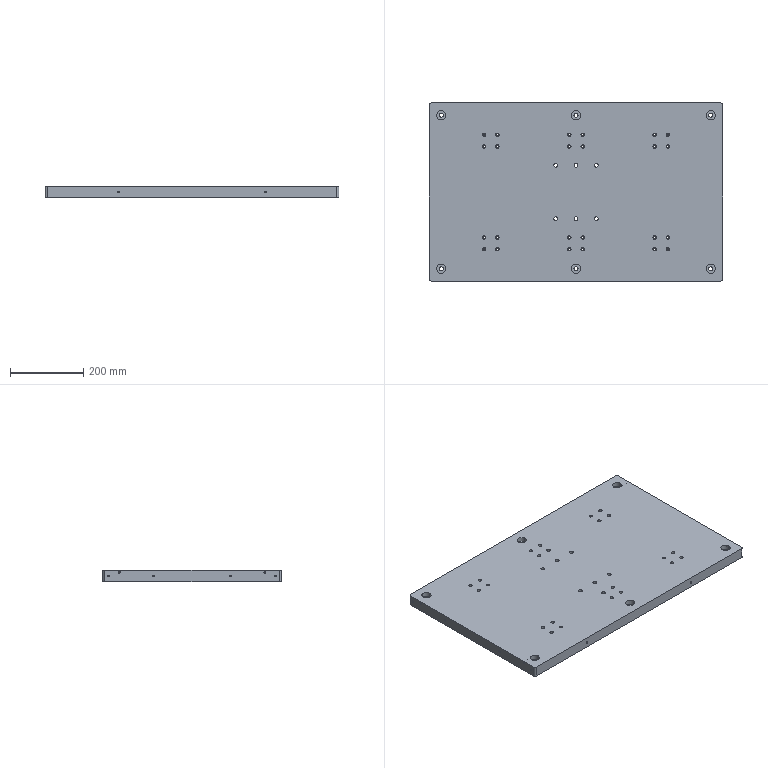CAM job | Mastercam | 3-axis milling, drilling | part box 800 x 485 x 30 mm
Tools:
tool_number,name,type,diameter_mm,corner_radius_mm,flutes,flute_length_mm,overall_length_mm,shoulder_length_mm,holder_diameter_mm,length_offset,diameter_offset,default_rpm,default_feed_mm_min,default_plunge_mm_min,coolant
1,11 Drill,drill,11,0,2,25,50,40,50,1,1,545,65.4,600,COOL_OFF
1,6.8 Drill,drill,6.8,0,2,25,50,40,50,1,1,1500,200,600,COOL_OFF
1,11 Drill,drill,11,0,2,25,50,40,50,1,1,545,65.4,600,COOL_OFF
1,11 Drill,drill,11,0,2,25,50,40,50,1,1,545,65.4,600,COOL_OFF
1,10 Drill,drill,10,0,2,25,50,40,50,1,1,600,72,600,COOL_OFF
5,5 Flat End Mill,end mill,5,0,4,25,75,25,50,5,5,2000,240,600,COOL_OFF
7,4 Chamfer Mill,chamfer mill,4,0,4,25,75,30,50,7,7,6250,750,600,COOL_OFF
7,6 Chamfer Mill,chamfer mill,6,0,4,25,75,30,50,7,7,7000,1000,600,COOL_OFF
7,4 Chamfer Mill,chamfer mill,4,0,4,25,75,30,50,7,7,6250,750,600,COOL_OFF
7,4 Chamfer Mill,chamfer mill,4,0,4,25,75,30,50,7,7,6250,750,600,COOL_OFF
9,10 Flat End Mill,end mill,10,0,4,25,75,25,50,9,9,1000,120,600,COOL_OFF
9,10 Flat End Mill,end mill,10,0,4,25,75,25,50,9,9,7000,3000,600,COOL_OFF
9,10 Flat End Mill,end mill,10,0,4,25,75,25,50,9,9,1000,120,600,COOL_OFF
9,10 Flat End Mill,end mill,10,0,4,25,75,25,50,9,9,1000,120,600,COOL_OFF
10,10 Flat End Mill,end mill,10,0,4,25,75,25,50,10,10,1000,120,600,COOL_OFF
10,10 Flat End Mill,end mill,10,0,4,25,75,25,50,10,10,1000,120,600,COOL_OFF
10,10 Flat End Mill,end mill,10,0,4,25,75,25,50,10,10,7000,1000,600,COOL_OFF
10,10 Flat End Mill,end mill,10,0,4,25,75,25,50,10,10,1000,120,600,COOL_OFF
14,10.5 Drill,drill,10.5,0,2,25,50,40,50,14,14,571,68.52,600,COOL_OFF
14,10.5 Drill,drill,10.5,0,2,25,50,40,50,14,14,571,68.52,600,COOL_OFF
14,10.5 Drill,drill,10.5,0,2,25,50,40,50,14,14,571,68.52,600,COOL_OFF
15,5.5 Drill,drill,5.5,0,2,25,50,40,50,15,15,1091,130.92,600,COOL_OFF
18,8 Drill,drill,8,0,2,25,50,40,50,18,18,1400,200,600,COOL_OFF
18,5.1 Drill,drill,5.1,0,2,25,50,40,50,18,18,1176,141.12,600,COOL_OFF
18,5.1 Drill,drill,5.1,0,2,25,50,40,50,18,18,1176,141.12,600,COOL_OFF
18,8.5 Drill,drill,8.5,0,2,25,50,40,50,18,18,706,84.72,600,COOL_OFF
19,9 Drill,drill,9,0,2,25,50,40,50,19,19,666,79.92,600,COOL_OFF
20,20 Flat End Mill,end mill,20,0,4,25,75,25,50,20,20,500,60,600,COOL_OFF
20,20 Flat End Mill,end mill,20,0,4,25,75,25,50,20,20,5000,4000,600,COOL_OFF
20,20 Flat End Mill,end mill,20,0,4,25,75,25,50,20,20,500,60,600,COOL_OFF
20,20 Flat End Mill,end mill,20,0,4,25,75,25,50,20,20,500,60,600,COOL_OFF
24,100 Flat End Mill,end mill,100,0,4,25,75,25,50,24,24,100,12,600,COOL_OFF
Operations:
seq,operation,operation_type,tool_number,tool_name,tool_diameter_mm,spindle_rpm,feed_mm_min,plunge_mm_min,retract_mm_min,cycle_time_s,wcs,posted,nc_file
1,Manual Entry (clamp x),ManualEntry,,,,0,0,0,0,0,Plane-1,yes,1.nc
2,Contour (Ramp) - [WCS: Plane-1] - [Tplane: Plane-1],Contour,20,20 Flat End Mill,20,5000,4000,600,1200,754.428,Plane-1,yes,1.nc
3,Contour (2D) - [WCS: Plane-1] - [Tplane: Plane-1],Contour,20,20 Flat End Mill,20,5000,1000,600,1200,221.553,Plane-1,yes,1.nc
4,Contour (2D chamfer) - [WCS: Plane-1] - [Tplane: Plane-1],Contour,7,4 Chamfer Mill,4,6500,1000,600,1200,98.508,Plane-1,yes,1.nc
5,Manual Entry (cCl，cy),ManualEntry,,,,0,0,0,0,0,Plane-1,yes,1.nc
6,Manual Entry (M00),ManualEntry,,,,0,0,0,0,0,Plane-1,yes,1.nc
7,Contour (Ramp) - [WCS: Plane-1] - [Tplane: Plane-1],Contour,20,20 Flat End Mill,20,5000,4000,600,1200,486.877,Plane-1,yes,1.nc
8,Contour (2D) - [WCS: Plane-1] - [Tplane: Plane-1],Contour,20,20 Flat End Mill,20,5000,1000,600,1200,147.1,Plane-1,yes,1.nc
9,Contour (2D chamfer) - [WCS: Plane-1] - [Tplane: Plane-1],Contour,7,4 Chamfer Mill,4,6500,1000,600,1200,60.684,Plane-1,yes,1.nc
10,Manual Entry (X+Cl),ManualEntry,,,,0,0,0,0,0,Plane-1,yes,1.nc
11,Manual Entry (M00),ManualEntry,,,,0,0,0,0,0,Plane-1,yes,1.nc
12,Drill/Counterbore - [WCS: Plane-1] - [Tplane: Plane-1],Drill,7,4 Chamfer Mill,4,6000,200,600,1200,35.588,Plane-1,yes,1.nc
13,Peck Drill - [WCS: Plane-1] - [Tplane: Plane-1],Drill,1,10 Drill,10,800,80,600,1200,156.133,Plane-1,yes,1.nc
14,Peck Drill - [WCS: Plane-1] - [Tplane: Plane-1],Drill,15,5.5 Drill,5.5,1200,120,600,1200,439.734,Plane-1,yes,1.nc
15,Peck Drill - [WCS: Plane-1] - [Tplane: Plane-1],Drill,14,10.5 Drill,10.5,800,100,600,1200,128.413,Plane-1,yes,1.nc
16,Helix Bore - [WCS: Plane-1] - [Tplane: Plane-1],HelixBore,5,5 Flat End Mill,5,6500,2000,600,1200,485.706,Plane-1,yes,1.nc
17,Contour (Ramp) - [WCS: Plane-1] - [Tplane: Plane-1],Contour,9,10 Flat End Mill,10,6500,3000,600,1200,113.28,Plane-1,yes,1.nc
18,Contour (2D) - [WCS: Plane-1] - [Tplane: Plane-1],Contour,10,10 Flat End Mill,10,6500,1000,600,1200,59.619,Plane-1,yes,1.nc
19,Contour (2D chamfer) - [WCS: Plane-1] - [Tplane: Plane-1],Contour,7,4 Chamfer Mill,4,6000,1000,600,1200,116.625,Plane-1,yes,1.nc
20,Contour (Ramp) - [WCS: Plane-2] - [Tplane: Plane-2],Contour,9,10 Flat End Mill,10,6500,2000,600,1200,80.577,Plane-2,yes,1.nc
21,Contour (2D) - [WCS: Plane-2] - [Tplane: Plane-2],Contour,10,10 Flat End Mill,10,6500,1000,600,1200,19.005,Plane-2,yes,1.nc
22,Contour (2D chamfer) - [WCS: Plane-2] - [Tplane: Plane-2],Contour,7,4 Chamfer Mill,4,6000,1000,600,1200,37.556,Plane-2,yes,1.nc
23,Drill/Counterbore - [WCS: Plane-3] - [Tplane: Plane-3],Drill,7,4 Chamfer Mill,4,6000,200,600,1200,1.977,Plane-3,yes,1.nc
24,Peck Drill - [WCS: Plane-3] - [Tplane: Plane-3],Drill,18,8.5 Drill,8.5,1200,100,600,1200,31.296,Plane-3,yes,1.nc
25,Contour (2D chamfer) - [WCS: Plane-3] - [Tplane: Plane-3],Contour,7,4 Chamfer Mill,4,6000,1000,600,1200,3.002,Plane-3,yes,1.nc
26,Drill/Counterbore - [WCS: Plane-4] - [Tplane: Plane-4],Drill,7,4 Chamfer Mill,4,6000,200,600,1200,5.931,Plane-4,yes,1.nc
27,Peck Drill - [WCS: Plane-4] - [Tplane: Plane-4],Drill,15,5.5 Drill,5.5,1200,100,600,1200,85.363,Plane-4,yes,1.nc
28,Contour (2D chamfer) - [WCS: Plane-4] - [Tplane: Plane-4],Contour,7,4 Chamfer Mill,4,6000,1000,600,1200,9.231,Plane-4,yes,1.nc
29,Contour (Ramp) - [WCS: Plane-2] - [Tplane: Plane-2],Contour,10,10 Flat End Mill,10,6500,1500,600,1200,29.736,Plane-2,yes,1.nc
30,Manual Entry (clamp x),ManualEntry,,,,0,0,0,0,0,Plane-5,yes,4.nc
31,Contour (Ramp) - [WCS: Plane-5] - [Tplane: Plane-5],Contour,20,20 Flat End Mill,20,5000,4000,600,1200,628.88,Plane-5,yes,4.nc
32,Contour (2D) - [WCS: Plane-5] - [Tplane: Plane-5],Contour,20,20 Flat End Mill,20,5000,1000,600,1200,219.457,Plane-5,yes,4.nc
33,Contour (2D chamfer) - [WCS: Plane-5] - [Tplane: Plane-5],Contour,7,4 Chamfer Mill,4,6500,1000,600,1200,98.508,Plane-5,yes,4.nc
34,Manual Entry (cCl，cy),ManualEntry,,,,0,0,0,0,0,Plane-5,yes,4.nc
35,Manual Entry (M00),ManualEntry,,,,0,0,0,0,0,Plane-5,yes,4.nc
36,Contour (Ramp) - [WCS: Plane-5] - [Tplane: Plane-5],Contour,20,20 Flat End Mill,20,5000,4000,600,1200,405.921,Plane-5,yes,4.nc
37,Contour (2D) - [WCS: Plane-5] - [Tplane: Plane-5],Contour,20,20 Flat End Mill,20,5000,1000,600,1200,145.004,Plane-5,yes,4.nc
38,Contour (2D chamfer) - [WCS: Plane-5] - [Tplane: Plane-5],Contour,7,4 Chamfer Mill,4,6500,1000,600,1200,60.684,Plane-5,yes,4.nc
39,Manual Entry (M00),ManualEntry,,,,0,0,0,0,0,Plane-5,yes,4.nc
40,Manual Entry (x+Cl),ManualEntry,,,,0,0,0,0,0,Plane-5,yes,4.nc
41,Contour (Ramp) - [WCS: Plane-5] - [Tplane: Plane-5],Contour,20,20 Flat End Mill,20,4000,3000,600,1200,518.461,Plane-5,yes,4.nc
42,Drill/Counterbore - [WCS: Plane-5] - [Tplane: Plane-5],Drill,7,4 Chamfer Mill,4,3000,300,600,1200,24.557,Plane-5,yes,4.nc
43,Peck Drill - [WCS: Plane-5] - [Tplane: Plane-5],Drill,1,10 Drill,10,800,100,600,1200,105.431,Plane-5,yes,4.nc
44,Peck Drill - [WCS: Plane-5] - [Tplane: Plane-5],Drill,14,10.5 Drill,10.5,800,100,600,1200,421.724,Plane-5,yes,4.nc
45,Contour (Ramp) - [WCS: Plane-5] - [Tplane: Plane-5],Contour,9,10 Flat End Mill,10,6500,3500,600,1200,72.475,Plane-5,yes,4.nc
46,Contour (2D) - [WCS: Plane-5] - [Tplane: Plane-5],Contour,10,10 Flat End Mill,10,6500,1000,600,1200,41.967,Plane-5,yes,4.nc
47,Contour (2D) - [WCS: Plane-5] - [Tplane: Plane-5],Contour,10,10 Flat End Mill,10,6500,1000,600,1200,126.936,Plane-5,yes,4.nc
48,Contour (2D chamfer) - [WCS: Plane-5] - [Tplane: Plane-5],Contour,7,4 Chamfer Mill,4,6000,1000,600,1200,174.87,Plane-5,yes,4.nc
49,Drill/Counterbore - [WCS: Plane-6] - [Tplane: Plane-6],Drill,7,4 Chamfer Mill,4,6000,200,600,1200,1.977,Plane-6,yes,4.nc
50,Peck Drill - [WCS: Plane-6] - [Tplane: Plane-6],Drill,18,8.5 Drill,8.5,1200,120,600,1200,26.696,Plane-6,yes,4.nc
51,Contour (2D chamfer) - [WCS: Plane-6] - [Tplane: Plane-6],Contour,7,4 Chamfer Mill,4,6000,1000,600,1200,3.077,Plane-6,yes,4.nc
52,Drill/Counterbore - [WCS: Plane-7] - [Tplane: Plane-7],Drill,7,4 Chamfer Mill,4,6000,200,600,1200,2.966,Plane-7,yes,4.nc
53,Peck Drill - [WCS: Plane-7] - [Tplane: Plane-7],Drill,18,8.5 Drill,8.5,1200,120,600,1200,40.044,Plane-7,yes,4.nc
54,Contour (2D chamfer) - [WCS: Plane-7] - [Tplane: Plane-7],Contour,7,4 Chamfer Mill,4,6000,1000,600,1200,4.616,Plane-7,yes,4.nc
55,Manual Entry (clamp x),ManualEntry,,,,0,0,0,0,0,Plane-8,yes,2.nc
56,Contour (Ramp) - [WCS: Plane-8] - [Tplane: Plane-8],Contour,20,20 Flat End Mill,20,5000,4000,600,1200,621.38,Plane-8,yes,2.nc
57,Contour (2D) - [WCS: Plane-8] - [Tplane: Plane-8],Contour,20,20 Flat End Mill,20,5000,1000,600,1200,216.961,Plane-8,yes,2.nc
58,Contour (2D chamfer) - [WCS: Plane-8] - [Tplane: Plane-8],Contour,7,4 Chamfer Mill,4,6500,1200,600,1200,80.108,Plane-8,yes,2.nc
59,Manual Entry (cClcy),ManualEntry,,,,0,0,0,0,0,Plane-8,yes,2.nc
60,Manual Entry (M00),ManualEntry,,,,0,0,0,0,0,Plane-8,yes,2.nc
61,Contour (Ramp) - [WCS: Plane-8] - [Tplane: Plane-8],Contour,20,20 Flat End Mill,20,5000,4000,600,1200,322.671,Plane-8,yes,2.nc
62,Contour (2D) - [WCS: Plane-8] - [Tplane: Plane-8],Contour,20,20 Flat End Mill,20,5000,1000,600,1200,117.298,Plane-8,yes,2.nc
63,Contour (2D chamfer) - [WCS: Plane-8] - [Tplane: Plane-8],Contour,7,4 Chamfer Mill,4,6500,1000,600,1200,46.98,Plane-8,yes,2.nc
64,Drill/Counterbore - [WCS: Plane-8] - [Tplane: Plane-8],Drill,7,4 Chamfer Mill,4,6000,200,600,1200,19.771,Plane-8,yes,2.nc
65,Peck Drill - [WCS: Plane-8] - [Tplane: Plane-8],Drill,19,9 Drill,9,800,100,600,1200,140.575,Plane-8,yes,2.nc
66,Peck Drill - [WCS: Plane-8] - [Tplane: Plane-8],Drill,18,8.5 Drill,8.5,800,100,600,1200,210.862,Plane-8,yes,2.nc
67,Contour (2D chamfer) - [WCS: Plane-8] - [Tplane: Plane-8],Contour,7,4 Chamfer Mill,4,6500,1200,600,1200,39.662,Plane-8,yes,2.nc
68,Drill/Counterbore - [WCS: Plane-9] - [Tplane: Plane-9],Drill,7,4 Chamfer Mill,4,6000,200,600,1200,7.908,Plane-9,yes,2.nc
69,Peck Drill - [WCS: Plane-9] - [Tplane: Plane-9],Drill,1,10 Drill,10,800,80,600,1200,271.231,Plane-9,yes,2.nc
70,Peck Drill - [WCS: Plane-9] - [Tplane: Plane-9],Drill,14,10.5 Drill,10.5,800,80,600,1200,43.186,Plane-9,yes,2.nc
71,Contour (2D chamfer) - [WCS: Plane-9] - [Tplane: Plane-9],Contour,7,4 Chamfer Mill,4,6500,1200,600,1200,17.505,Plane-9,yes,2.nc
72,Manual Entry (LRre),ManualEntry,,,,0,0,0,0,0,Plane-11,yes,3.nc
73,Contour (Ramp) - [WCS: Plane-11] - [Tplane: Plane-10],Contour,9,10 Flat End Mill,10,7000,3000,600,1200,661.332,Plane-11,yes,3.nc
74,Contour (2D) - [WCS: Plane-11] - [Tplane: Plane-10],Contour,10,10 Flat End Mill,10,7000,1000,600,1200,103.732,Plane-11,yes,3.nc
75,Contour (2D chamfer) - [WCS: Plane-11] - [Tplane: Plane-10],Contour,7,4 Chamfer Mill,4,7000,1000,600,1200,99.718,Plane-11,yes,3.nc
76,Manual Entry (LRrecFRbl),ManualEntry,,,,0,0,0,0,0,Plane-11,yes,3.nc
77,Contour (Ramp) - [WCS: Plane-11] - [Tplane: Plane-10],Contour,9,10 Flat End Mill,10,7000,3000,600,1200,311.194,Plane-11,yes,3.nc
78,Contour (2D) - [WCS: Plane-11] - [Tplane: Plane-10],Contour,10,10 Flat End Mill,10,7000,1000,600,1200,51.136,Plane-11,yes,3.nc
79,2D High Speed (2D Area Mill) - [WCS: Plane-11] - [Tplane: Plane-10],HighSpeed2D,20,20 Flat End Mill,20,5000,4000,600,1200,1013.835,Plane-11,yes,3.nc
80,Contour (Remachining) - [WCS: Plane-11] - [Tplane: Plane-10],Contour,9,10 Flat End Mill,10,7000,3000,600,1200,78.027,Plane-11,yes,3.nc
81,2D High Speed (2D Area Mill) - [WCS: Plane-11] - [Tplane: Plane-10],HighSpeed2D,10,10 Flat End Mill,10,7000,1000,600,1200,1084.986,Plane-11,yes,3.nc
82,Contour (2D) - [WCS: Plane-11] - [Tplane: Plane-10],Contour,10,10 Flat End Mill,10,7000,1000,600,1200,195.666,Plane-11,yes,3.nc
83,2D High Speed (2D Area Rest Mill) - [WCS: Plane-11] - [Tplane: Plane-10],HighSpeed2D,9,10 Flat End Mill,10,7000,3000,600,1200,2177.69,Plane-11,yes,3.nc
84,2D High Speed (2D Area Rest Mill) - [WCS: Plane-11] - [Tplane: Plane-10],HighSpeed2D,10,10 Flat End Mill,10,7000,1000,600,1200,1233.522,Plane-11,yes,3.nc
85,Contour (2D) - [WCS: Plane-11] - [Tplane: Plane-10],Contour,10,10 Flat End Mill,10,7000,1000,600,1200,119.884,Plane-11,yes,3.nc
86,Drill/Counterbore - [WCS: Plane-11] - [Tplane: Plane-10],Drill,7,4 Chamfer Mill,4,7000,1000,600,1200,14.563,Plane-11,yes,3.nc
87,Peck Drill - [WCS: Plane-11] - [Tplane: Plane-10],Drill,1,10 Drill,10,1500,200,600,1200,45.014,Plane-11,yes,3.nc
88,Peck Drill - [WCS: Plane-11] - [Tplane: Plane-10],Drill,18,8.5 Drill,8.5,1400,200,600,1200,58.478,Plane-11,yes,3.nc
89,Model Chamfer - [WCS: Plane-11] - [Tplane: Plane-10],ModelChamfer,7,4 Chamfer Mill,4,7000,1000,600,1200,423.579,Plane-11,yes,3.nc
90,Contour (2D) - [WCS: Plane-11] - [Tplane: Plane-10],Contour,24,100 Flat End Mill,100,4000,1000,600,1200,115.731,Plane-11,yes,3.nc
91,Manual Entry (Front Rear blue chamfer red 加黄色),ManualEntry,,,,0,0,0,0,0,Plane-11,yes,3.nc
92,Contour (2D) - [WCS: Plane-11] - [Tplane: Plane-10],Contour,9,10 Flat End Mill,10,7000,3000,600,1200,187.78,Plane-11,yes,3.nc
93,Contour (2D) - [WCS: Plane-11] - [Tplane: Plane-10],Contour,10,10 Flat End Mill,10,7000,1000,600,1200,108.804,Plane-11,yes,3.nc